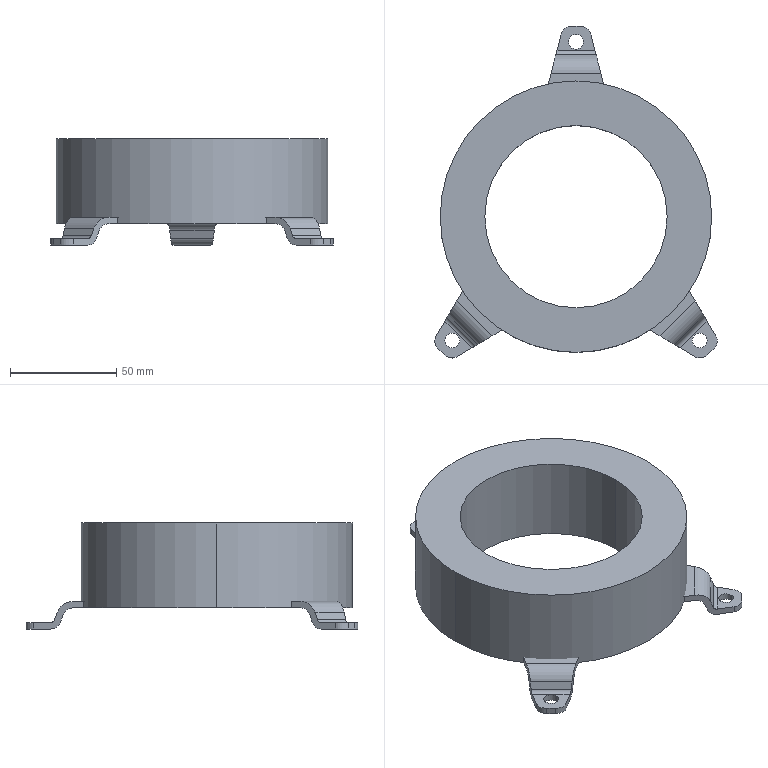Part | STEP file | 10P30 stator | 4 solids | 67 faces | box 133.205 x 156.603 x 50 mm | volume 289241 mm3 | plane 38 | cylinder 29 | commonest cylinder face diameters 10 x13 7 x6 4 x3 16 x3 86 x2 128 x2